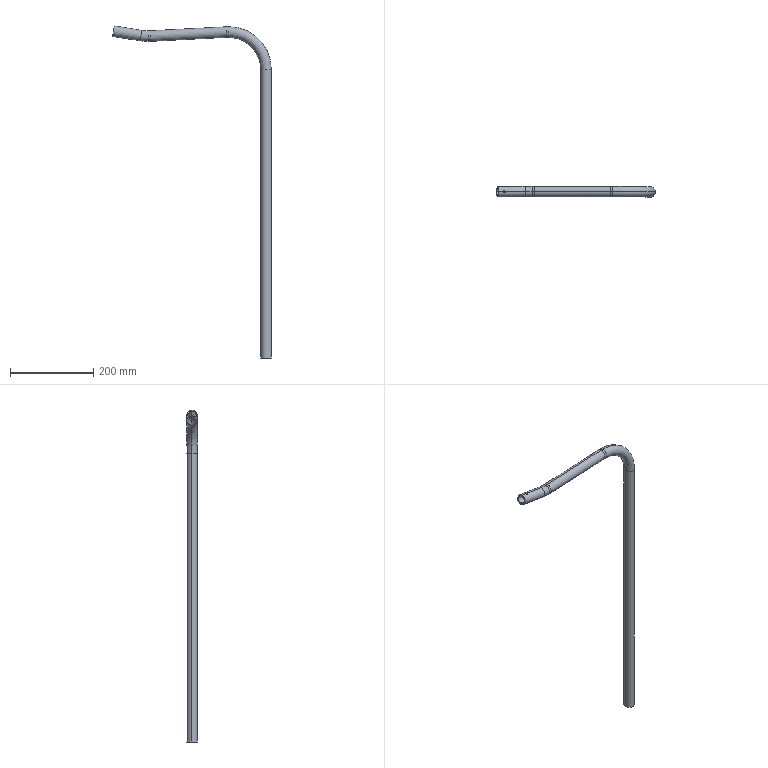Part | STEP file | PN_0029_Default<As Machined> | 1 solid | 38 faces | box 380.934 x 25.4 x 797.47 mm | volume 220981 mm3 | cylinder 16 | torus 16 | cone 4 | plane 2 | commonest cylinder face diameters 19.8 x6 25.4 x6 4.2 x4
STEP:
#1=CARTESIAN_POINT('',(-19.357,0.,-635.525));
#2=VERTEX_POINT('',#1);
#3=CARTESIAN_POINT('',(-18.145,-1.843,-634.518));
#4=VERTEX_POINT('',#3);
#5=CARTESIAN_POINT('',(-18.751,-0.9215,-635.022));
#6=DIRECTION('',(0.5,-0.76,0.4152));
#7=VECTOR('',#6,1.);
#8=LINE('',#5,#7);
#9=EDGE_CURVE('',#2,#4,#8,.T.);
#10=ORIENTED_EDGE('',*,*,#9,.T.);
#11=CARTESIAN_POINT('',(-18.145,1.843,-636.532));
#12=VERTEX_POINT('',#11);
#13=CARTESIAN_POINT('',(-18.145,0.,-635.525));
#14=DIRECTION('',(1.,0.,0.));
#15=AXIS2_PLACEMENT_3D('',#13,#14,$);
#16=CIRCLE('',#15,2.1);
#17=EDGE_CURVE('',#12,#4,#16,.F.);
#18=ORIENTED_EDGE('',*,*,#17,.F.);
#19=CARTESIAN_POINT('',(-18.751,0.9215,-636.028));
#20=DIRECTION('',(0.5,0.76,-0.4152));
#21=VECTOR('',#20,1.);
#22=LINE('',#19,#21);
#23=EDGE_CURVE('',#2,#12,#22,.T.);
#24=ORIENTED_EDGE('',*,*,#23,.F.);
#25=EDGE_LOOP('',(#10,#18,#24));
#26=FACE_OUTER_BOUND('',#25,.T.);
#27=CARTESIAN_POINT('',(-19.357,0.,-635.525));
#28=DIRECTION('',(1.,0.,0.));
#29=DIRECTION('',(0.,0.8776,-0.4794));
#30=AXIS2_PLACEMENT_3D('',#27,#28,#29);
#31=CONICAL_SURFACE('',#30,0.,1.047);
#32=ADVANCED_FACE('',(#26),#31,.F.);
#33=CARTESIAN_POINT('',(-17.145,0.,37.475));
#34=VERTEX_POINT('',#33);
#35=CARTESIAN_POINT('',(-17.145,0.,-633.425));
#36=VERTEX_POINT('',#35);
#37=CARTESIAN_POINT('',(-17.145,0.,37.475));
#38=DIRECTION('',(0.,0.,-1.));
#39=VECTOR('',#38,1.);
#40=LINE('',#37,#39);
#41=EDGE_CURVE('',#34,#36,#40,.T.);
#42=ORIENTED_EDGE('',*,*,#41,.F.);
#43=CARTESIAN_POINT('',(-42.545,0.,37.475));
#44=VERTEX_POINT('',#43);
#45=CARTESIAN_POINT('',(-29.845,0.,37.475));
#46=DIRECTION('',(0.,0.,-1.));
#47=AXIS2_PLACEMENT_3D('',#45,#46,$);
#48=CIRCLE('',#47,12.7);
#49=EDGE_CURVE('',#34,#44,#48,.T.);
#50=ORIENTED_EDGE('',*,*,#49,.T.);
#51=CARTESIAN_POINT('',(-42.545,0.,-655.525));
#52=VERTEX_POINT('',#51);
#53=CARTESIAN_POINT('',(-42.545,0.,37.475));
#54=DIRECTION('',(0.,0.,-1.));
#55=VECTOR('',#54,1.);
#56=LINE('',#53,#55);
#57=EDGE_CURVE('',#44,#52,#56,.T.);
#58=ORIENTED_EDGE('',*,*,#57,.T.);
#59=CARTESIAN_POINT('',(-17.145,0.,-655.525));
#60=VERTEX_POINT('',#59);
#61=CARTESIAN_POINT('',(-29.845,0.,-655.525));
#62=DIRECTION('',(0.,0.,-1.));
#63=AXIS2_PLACEMENT_3D('',#61,#62,$);
#64=CIRCLE('',#63,12.7);
#65=EDGE_CURVE('',#60,#52,#64,.T.);
#66=ORIENTED_EDGE('',*,*,#65,.F.);
#67=CARTESIAN_POINT('',(-17.145,0.,-637.625));
#68=VERTEX_POINT('',#67);
#69=CARTESIAN_POINT('',(-17.145,0.,37.475));
#70=DIRECTION('',(0.,0.,-1.));
#71=VECTOR('',#70,1.);
#72=LINE('',#69,#71);
#73=EDGE_CURVE('',#68,#60,#72,.T.);
#74=ORIENTED_EDGE('',*,*,#73,.F.);
#75=CARTESIAN_POINT('',(-17.279,-1.843,-634.518));
#76=VERTEX_POINT('',#75);
#77=CARTESIAN_POINT('',(-17.279,-1.843,-634.518));
#78=CARTESIAN_POINT('',(-17.34,-2.259,-635.281));
#79=CARTESIAN_POINT('',(-17.369,-2.286,-636.267));
#80=CARTESIAN_POINT('',(-17.221,-1.743,-637.175));
#81=CARTESIAN_POINT('',(-17.145,-0.871,-637.625));
#82=CARTESIAN_POINT('',(-17.145,0.,-637.625));
#83=B_SPLINE_CURVE_WITH_KNOTS('',5,(#77,#78,#79,#80,#81,#82),.UNSPECIFIED.,.F.,.U.,(6,6),(0.,6.159),.UNSPECIFIED.);
#84=EDGE_CURVE('',#76,#68,#83,.T.);
#85=ORIENTED_EDGE('',*,*,#84,.F.);
#86=CARTESIAN_POINT('',(-17.279,-1.843,-634.518));
#87=CARTESIAN_POINT('',(-17.24,-1.574,-634.025));
#88=CARTESIAN_POINT('',(-17.18,-1.128,-633.628));
#89=CARTESIAN_POINT('',(-17.145,-0.5633,-633.425));
#90=CARTESIAN_POINT('',(-17.145,0.,-633.425));
#91=B_SPLINE_CURVE_WITH_KNOTS('',4,(#86,#87,#88,#89,#90),.UNSPECIFIED.,.F.,.U.,(5,5),(0.,3.187),.UNSPECIFIED.);
#92=EDGE_CURVE('',#76,#36,#91,.T.);
#93=ORIENTED_EDGE('',*,*,#92,.T.);
#94=EDGE_LOOP('',(#42,#50,#58,#66,#74,#85,#93));
#95=FACE_OUTER_BOUND('',#94,.T.);
#96=CARTESIAN_POINT('',(-29.845,0.,37.475));
#97=DIRECTION('',(0.,0.,-1.));
#98=DIRECTION('',(1.,0.,0.));
#99=AXIS2_PLACEMENT_3D('',#96,#97,#98);
#100=CYLINDRICAL_SURFACE('',#99,12.7);
#101=ADVANCED_FACE('',(#95),#100,.T.);
#102=CARTESIAN_POINT('',(-119.845,0.,140.175));
#103=VERTEX_POINT('',#102);
#104=CARTESIAN_POINT('',(-119.845,0.,37.475));
#105=DIRECTION('',(0.,1.,0.));
#106=AXIS2_PLACEMENT_3D('',#104,#105,$);
#107=CIRCLE('',#106,102.7);
#108=EDGE_CURVE('',#103,#34,#107,.T.);
#109=ORIENTED_EDGE('',*,*,#108,.F.);
#110=CARTESIAN_POINT('',(-119.845,0.,114.775));
#111=VERTEX_POINT('',#110);
#112=CARTESIAN_POINT('',(-119.845,0.,127.475));
#113=DIRECTION('',(-1.,0.,0.));
#114=AXIS2_PLACEMENT_3D('',#112,#113,$);
#115=CIRCLE('',#114,12.7);
#116=EDGE_CURVE('',#111,#103,#115,.T.);
#117=ORIENTED_EDGE('',*,*,#116,.F.);
#118=CARTESIAN_POINT('',(-119.845,0.,37.475));
#119=DIRECTION('',(0.,1.,0.));
#120=AXIS2_PLACEMENT_3D('',#118,#119,$);
#121=CIRCLE('',#120,77.3);
#122=EDGE_CURVE('',#111,#44,#121,.T.);
#123=ORIENTED_EDGE('',*,*,#122,.T.);
#124=ORIENTED_EDGE('',*,*,#49,.F.);
#125=EDGE_LOOP('',(#109,#117,#123,#124));
#126=FACE_OUTER_BOUND('',#125,.T.);
#127=CARTESIAN_POINT('',(-119.845,0.,37.475));
#128=DIRECTION('',(0.,1.,0.));
#129=DIRECTION('',(0.,0.,1.));
#130=AXIS2_PLACEMENT_3D('',#127,#128,#129);
#131=TOROIDAL_SURFACE('',#130,90.,12.7);
#132=ADVANCED_FACE('',(#126),#131,.T.);
#133=CARTESIAN_POINT('',(-39.745,0.,37.475));
#134=VERTEX_POINT('',#133);
#135=CARTESIAN_POINT('',(-19.945,0.,37.475));
#136=VERTEX_POINT('',#135);
#137=CARTESIAN_POINT('',(-29.845,0.,37.475));
#138=DIRECTION('',(0.,0.,-1.));
#139=AXIS2_PLACEMENT_3D('',#137,#138,$);
#140=CIRCLE('',#139,9.9);
#141=EDGE_CURVE('',#134,#136,#140,.F.);
#142=ORIENTED_EDGE('',*,*,#141,.T.);
#143=CARTESIAN_POINT('',(-19.945,0.,-655.525));
#144=VERTEX_POINT('',#143);
#145=CARTESIAN_POINT('',(-19.945,0.,37.475));
#146=DIRECTION('',(0.,0.,-1.));
#147=VECTOR('',#146,1.);
#148=LINE('',#145,#147);
#149=EDGE_CURVE('',#136,#144,#148,.T.);
#150=ORIENTED_EDGE('',*,*,#149,.T.);
#151=CARTESIAN_POINT('',(-39.745,0.,-655.525));
#152=VERTEX_POINT('',#151);
#153=CARTESIAN_POINT('',(-29.845,0.,-655.525));
#154=DIRECTION('',(0.,0.,-1.));
#155=AXIS2_PLACEMENT_3D('',#153,#154,$);
#156=CIRCLE('',#155,9.9);
#157=EDGE_CURVE('',#152,#144,#156,.F.);
#158=ORIENTED_EDGE('',*,*,#157,.F.);
#159=CARTESIAN_POINT('',(-39.745,0.,37.475));
#160=DIRECTION('',(0.,0.,-1.));
#161=VECTOR('',#160,1.);
#162=LINE('',#159,#161);
#163=EDGE_CURVE('',#134,#152,#162,.T.);
#164=ORIENTED_EDGE('',*,*,#163,.F.);
#165=EDGE_LOOP('',(#142,#150,#158,#164));
#166=FACE_OUTER_BOUND('',#165,.T.);
#167=CARTESIAN_POINT('',(-29.845,0.,37.475));
#168=DIRECTION('',(0.,0.,-1.));
#169=DIRECTION('',(1.,0.,0.));
#170=AXIS2_PLACEMENT_3D('',#167,#168,#169);
#171=CYLINDRICAL_SURFACE('',#170,9.9);
#172=ADVANCED_FACE('',(#166),#171,.F.);
#173=ORIENTED_EDGE('',*,*,#149,.F.);
#174=CARTESIAN_POINT('',(-29.845,0.,37.475));
#175=DIRECTION('',(0.,0.,-1.));
#176=AXIS2_PLACEMENT_3D('',#174,#175,$);
#177=CIRCLE('',#176,9.9);
#178=EDGE_CURVE('',#136,#134,#177,.F.);
#179=ORIENTED_EDGE('',*,*,#178,.T.);
#180=ORIENTED_EDGE('',*,*,#163,.T.);
#181=CARTESIAN_POINT('',(-29.845,0.,-655.525));
#182=DIRECTION('',(0.,0.,-1.));
#183=AXIS2_PLACEMENT_3D('',#181,#182,$);
#184=CIRCLE('',#183,9.9);
#185=EDGE_CURVE('',#144,#152,#184,.F.);
#186=ORIENTED_EDGE('',*,*,#185,.F.);
#187=EDGE_LOOP('',(#173,#179,#180,#186));
#188=FACE_OUTER_BOUND('',#187,.T.);
#189=CARTESIAN_POINT('',(-29.845,0.,37.475));
#190=DIRECTION('',(0.,0.,-1.));
#191=DIRECTION('',(-1.,0.,0.));
#192=AXIS2_PLACEMENT_3D('',#189,#190,#191);
#193=CYLINDRICAL_SURFACE('',#192,9.9);
#194=ADVANCED_FACE('',(#188),#193,.F.);
#195=CARTESIAN_POINT('',(-119.845,0.,117.575));
#196=VERTEX_POINT('',#195);
#197=CARTESIAN_POINT('',(-119.845,0.,137.375));
#198=VERTEX_POINT('',#197);
#199=CARTESIAN_POINT('',(-119.845,0.,127.475));
#200=DIRECTION('',(-1.,0.,0.));
#201=AXIS2_PLACEMENT_3D('',#199,#200,$);
#202=CIRCLE('',#201,9.9);
#203=EDGE_CURVE('',#196,#198,#202,.T.);
#204=ORIENTED_EDGE('',*,*,#203,.T.);
#205=CARTESIAN_POINT('',(-119.845,0.,37.475));
#206=DIRECTION('',(0.,1.,0.));
#207=AXIS2_PLACEMENT_3D('',#205,#206,$);
#208=CIRCLE('',#207,99.9);
#209=EDGE_CURVE('',#198,#136,#208,.T.);
#210=ORIENTED_EDGE('',*,*,#209,.T.);
#211=ORIENTED_EDGE('',*,*,#141,.F.);
#212=CARTESIAN_POINT('',(-119.845,0.,37.475));
#213=DIRECTION('',(0.,1.,0.));
#214=AXIS2_PLACEMENT_3D('',#212,#213,$);
#215=CIRCLE('',#214,80.1);
#216=EDGE_CURVE('',#196,#134,#215,.T.);
#217=ORIENTED_EDGE('',*,*,#216,.F.);
#218=EDGE_LOOP('',(#204,#210,#211,#217));
#219=FACE_OUTER_BOUND('',#218,.T.);
#220=CARTESIAN_POINT('',(-119.845,0.,37.475));
#221=DIRECTION('',(0.,1.,0.));
#222=DIRECTION('',(0.,0.,1.));
#223=AXIS2_PLACEMENT_3D('',#220,#221,#222);
#224=TOROIDAL_SURFACE('',#223,90.,9.9);
#225=ADVANCED_FACE('',(#219),#224,.F.);
#226=ORIENTED_EDGE('',*,*,#209,.F.);
#227=CARTESIAN_POINT('',(-119.845,0.,127.475));
#228=DIRECTION('',(-1.,0.,0.));
#229=AXIS2_PLACEMENT_3D('',#227,#228,$);
#230=CIRCLE('',#229,9.9);
#231=EDGE_CURVE('',#198,#196,#230,.T.);
#232=ORIENTED_EDGE('',*,*,#231,.T.);
#233=ORIENTED_EDGE('',*,*,#216,.T.);
#234=ORIENTED_EDGE('',*,*,#178,.F.);
#235=EDGE_LOOP('',(#226,#232,#233,#234));
#236=FACE_OUTER_BOUND('',#235,.T.);
#237=CARTESIAN_POINT('',(-119.845,0.,37.475));
#238=DIRECTION('',(0.,1.,0.));
#239=DIRECTION('',(0.,0.,1.));
#240=AXIS2_PLACEMENT_3D('',#237,#238,#239);
#241=TOROIDAL_SURFACE('',#240,90.,9.9);
#242=ADVANCED_FACE('',(#236),#241,.F.);
#243=CARTESIAN_POINT('',(-124.037,0.,117.465));
#244=VERTEX_POINT('',#243);
#245=CARTESIAN_POINT('',(-125.073,0.,137.238));
#246=VERTEX_POINT('',#245);
#247=CARTESIAN_POINT('',(-124.555,0.,127.352));
#248=DIRECTION('',(-0.9986,0.,-0.05234));
#249=AXIS2_PLACEMENT_3D('',#247,#248,$);
#250=CIRCLE('',#249,9.9);
#251=EDGE_CURVE('',#244,#246,#250,.T.);
#252=ORIENTED_EDGE('',*,*,#251,.T.);
#253=CARTESIAN_POINT('',(-119.845,0.,37.475));
#254=DIRECTION('',(0.,1.,0.));
#255=AXIS2_PLACEMENT_3D('',#253,#254,$);
#256=CIRCLE('',#255,99.9);
#257=EDGE_CURVE('',#246,#198,#256,.T.);
#258=ORIENTED_EDGE('',*,*,#257,.T.);
#259=ORIENTED_EDGE('',*,*,#203,.F.);
#260=CARTESIAN_POINT('',(-119.845,0.,37.475));
#261=DIRECTION('',(0.,1.,0.));
#262=AXIS2_PLACEMENT_3D('',#260,#261,$);
#263=CIRCLE('',#262,80.1);
#264=EDGE_CURVE('',#244,#196,#263,.T.);
#265=ORIENTED_EDGE('',*,*,#264,.F.);
#266=EDGE_LOOP('',(#252,#258,#259,#265));
#267=FACE_OUTER_BOUND('',#266,.T.);
#268=CARTESIAN_POINT('',(-119.845,0.,37.475));
#269=DIRECTION('',(0.,1.,0.));
#270=DIRECTION('',(0.,0.,-1.));
#271=AXIS2_PLACEMENT_3D('',#268,#269,#270);
#272=TOROIDAL_SURFACE('',#271,90.,9.9);
#273=ADVANCED_FACE('',(#267),#272,.F.);
#274=ORIENTED_EDGE('',*,*,#257,.F.);
#275=CARTESIAN_POINT('',(-124.555,0.,127.352));
#276=DIRECTION('',(-0.9986,0.,-0.05234));
#277=AXIS2_PLACEMENT_3D('',#275,#276,$);
#278=CIRCLE('',#277,9.9);
#279=EDGE_CURVE('',#246,#244,#278,.T.);
#280=ORIENTED_EDGE('',*,*,#279,.T.);
#281=ORIENTED_EDGE('',*,*,#264,.T.);
#282=ORIENTED_EDGE('',*,*,#231,.F.);
#283=EDGE_LOOP('',(#274,#280,#281,#282));
#284=FACE_OUTER_BOUND('',#283,.T.);
#285=CARTESIAN_POINT('',(-119.845,0.,37.475));
#286=DIRECTION('',(0.,1.,0.));
#287=DIRECTION('',(0.,0.,-1.));
#288=AXIS2_PLACEMENT_3D('',#285,#286,#287);
#289=TOROIDAL_SURFACE('',#288,90.,9.9);
#290=ADVANCED_FACE('',(#284),#289,.F.);
#291=CARTESIAN_POINT('',(-306.794,0.,107.887));
#292=VERTEX_POINT('',#291);
#293=CARTESIAN_POINT('',(-307.83,0.,127.66));
#294=VERTEX_POINT('',#293);
#295=CARTESIAN_POINT('',(-307.312,0.,117.774));
#296=DIRECTION('',(0.9986,0.,0.05234));
#297=AXIS2_PLACEMENT_3D('',#295,#296,$);
#298=CIRCLE('',#297,9.9);
#299=EDGE_CURVE('',#292,#294,#298,.F.);
#300=ORIENTED_EDGE('',*,*,#299,.T.);
#301=CARTESIAN_POINT('',(-307.83,0.,127.66));
#302=DIRECTION('',(0.9986,0.,0.05234));
#303=VECTOR('',#302,1.);
#304=LINE('',#301,#303);
#305=EDGE_CURVE('',#294,#246,#304,.T.);
#306=ORIENTED_EDGE('',*,*,#305,.T.);
#307=ORIENTED_EDGE('',*,*,#251,.F.);
#308=CARTESIAN_POINT('',(-306.794,0.,107.887));
#309=DIRECTION('',(0.9986,0.,0.05234));
#310=VECTOR('',#309,1.);
#311=LINE('',#308,#310);
#312=EDGE_CURVE('',#292,#244,#311,.T.);
#313=ORIENTED_EDGE('',*,*,#312,.F.);
#314=EDGE_LOOP('',(#300,#306,#307,#313));
#315=FACE_OUTER_BOUND('',#314,.T.);
#316=CARTESIAN_POINT('',(-307.312,0.,117.774));
#317=DIRECTION('',(0.9986,0.,0.05234));
#318=DIRECTION('',(-0.05234,0.,0.9986));
#319=AXIS2_PLACEMENT_3D('',#316,#317,#318);
#320=CYLINDRICAL_SURFACE('',#319,9.9);
#321=ADVANCED_FACE('',(#315),#320,.F.);
#322=ORIENTED_EDGE('',*,*,#305,.F.);
#323=CARTESIAN_POINT('',(-307.312,0.,117.774));
#324=DIRECTION('',(0.9986,0.,0.05234));
#325=AXIS2_PLACEMENT_3D('',#323,#324,$);
#326=CIRCLE('',#325,9.9);
#327=EDGE_CURVE('',#294,#292,#326,.F.);
#328=ORIENTED_EDGE('',*,*,#327,.T.);
#329=ORIENTED_EDGE('',*,*,#312,.T.);
#330=ORIENTED_EDGE('',*,*,#279,.F.);
#331=EDGE_LOOP('',(#322,#328,#329,#330));
#332=FACE_OUTER_BOUND('',#331,.T.);
#333=CARTESIAN_POINT('',(-307.312,0.,117.774));
#334=DIRECTION('',(0.9986,0.,0.05234));
#335=DIRECTION('',(0.05234,0.,-0.9986));
#336=AXIS2_PLACEMENT_3D('',#333,#334,#335);
#337=CYLINDRICAL_SURFACE('',#336,9.9);
#338=ADVANCED_FACE('',(#332),#337,.F.);
#339=CARTESIAN_POINT('',(-313.069,0.,107.723));
#340=VERTEX_POINT('',#339);
#341=CARTESIAN_POINT('',(-313.069,0.,227.623));
#342=DIRECTION('',(0.,-1.,0.));
#343=AXIS2_PLACEMENT_3D('',#341,#342,$);
#344=CIRCLE('',#343,119.9);
#345=EDGE_CURVE('',#340,#292,#344,.T.);
#346=ORIENTED_EDGE('',*,*,#345,.F.);
#347=CARTESIAN_POINT('',(-313.069,0.,127.523));
#348=VERTEX_POINT('',#347);
#349=CARTESIAN_POINT('',(-313.069,0.,117.623));
#350=DIRECTION('',(-1.,0.,0.));
#351=AXIS2_PLACEMENT_3D('',#349,#350,$);
#352=CIRCLE('',#351,9.9);
#353=EDGE_CURVE('',#340,#348,#352,.T.);
#354=ORIENTED_EDGE('',*,*,#353,.T.);
#355=CARTESIAN_POINT('',(-313.069,0.,227.623));
#356=DIRECTION('',(0.,-1.,0.));
#357=AXIS2_PLACEMENT_3D('',#355,#356,$);
#358=CIRCLE('',#357,100.1);
#359=EDGE_CURVE('',#348,#294,#358,.T.);
#360=ORIENTED_EDGE('',*,*,#359,.T.);
#361=ORIENTED_EDGE('',*,*,#299,.F.);
#362=EDGE_LOOP('',(#346,#354,#360,#361));
#363=FACE_OUTER_BOUND('',#362,.T.);
#364=CARTESIAN_POINT('',(-313.069,0.,227.623));
#365=DIRECTION('',(0.,-1.,0.));
#366=DIRECTION('',(0.,0.,-1.));
#367=AXIS2_PLACEMENT_3D('',#364,#365,#366);
#368=TOROIDAL_SURFACE('',#367,110.,9.9);
#369=ADVANCED_FACE('',(#363),#368,.F.);
#370=CARTESIAN_POINT('',(-313.069,0.,117.623));
#371=DIRECTION('',(-1.,0.,0.));
#372=AXIS2_PLACEMENT_3D('',#370,#371,$);
#373=CIRCLE('',#372,9.9);
#374=EDGE_CURVE('',#348,#340,#373,.T.);
#375=ORIENTED_EDGE('',*,*,#374,.T.);
#376=ORIENTED_EDGE('',*,*,#345,.T.);
#377=ORIENTED_EDGE('',*,*,#327,.F.);
#378=ORIENTED_EDGE('',*,*,#359,.F.);
#379=EDGE_LOOP('',(#375,#376,#377,#378));
#380=FACE_OUTER_BOUND('',#379,.T.);
#381=CARTESIAN_POINT('',(-313.069,0.,227.623));
#382=DIRECTION('',(0.,-1.,0.));
#383=DIRECTION('',(0.,0.,-1.));
#384=AXIS2_PLACEMENT_3D('',#381,#382,#383);
#385=TOROIDAL_SURFACE('',#384,110.,9.9);
#386=ADVANCED_FACE('',(#380),#385,.F.);
#387=CARTESIAN_POINT('',(-331.825,0.,109.199));
#388=VERTEX_POINT('',#387);
#389=CARTESIAN_POINT('',(-313.069,0.,227.623));
#390=DIRECTION('',(0.,-1.,0.));
#391=AXIS2_PLACEMENT_3D('',#389,#390,$);
#392=CIRCLE('',#391,119.9);
#393=EDGE_CURVE('',#388,#340,#392,.T.);
#394=ORIENTED_EDGE('',*,*,#393,.F.);
#395=CARTESIAN_POINT('',(-328.728,0.,128.755));
#396=VERTEX_POINT('',#395);
#397=CARTESIAN_POINT('',(-330.276,0.,118.977));
#398=DIRECTION('',(-0.9877,0.,0.1564));
#399=AXIS2_PLACEMENT_3D('',#397,#398,$);
#400=CIRCLE('',#399,9.9);
#401=EDGE_CURVE('',#388,#396,#400,.T.);
#402=ORIENTED_EDGE('',*,*,#401,.T.);
#403=CARTESIAN_POINT('',(-313.069,0.,227.623));
#404=DIRECTION('',(0.,-1.,0.));
#405=AXIS2_PLACEMENT_3D('',#403,#404,$);
#406=CIRCLE('',#405,100.1);
#407=EDGE_CURVE('',#396,#348,#406,.T.);
#408=ORIENTED_EDGE('',*,*,#407,.T.);
#409=ORIENTED_EDGE('',*,*,#353,.F.);
#410=EDGE_LOOP('',(#394,#402,#408,#409));
#411=FACE_OUTER_BOUND('',#410,.T.);
#412=CARTESIAN_POINT('',(-313.069,0.,227.623));
#413=DIRECTION('',(0.,-1.,0.));
#414=DIRECTION('',(0.,0.,1.));
#415=AXIS2_PLACEMENT_3D('',#412,#413,#414);
#416=TOROIDAL_SURFACE('',#415,110.,9.9);
#417=ADVANCED_FACE('',(#411),#416,.F.);
#418=CARTESIAN_POINT('',(-330.276,0.,118.977));
#419=DIRECTION('',(-0.9877,0.,0.1564));
#420=AXIS2_PLACEMENT_3D('',#418,#419,$);
#421=CIRCLE('',#420,9.9);
#422=EDGE_CURVE('',#396,#388,#421,.T.);
#423=ORIENTED_EDGE('',*,*,#422,.T.);
#424=ORIENTED_EDGE('',*,*,#393,.T.);
#425=ORIENTED_EDGE('',*,*,#374,.F.);
#426=ORIENTED_EDGE('',*,*,#407,.F.);
#427=EDGE_LOOP('',(#423,#424,#425,#426));
#428=FACE_OUTER_BOUND('',#427,.T.);
#429=CARTESIAN_POINT('',(-313.069,0.,227.623));
#430=DIRECTION('',(0.,-1.,0.));
#431=DIRECTION('',(0.,0.,1.));
#432=AXIS2_PLACEMENT_3D('',#429,#430,#431);
#433=TOROIDAL_SURFACE('',#432,110.,9.9);
#434=ADVANCED_FACE('',(#428),#433,.F.);
#435=CARTESIAN_POINT('',(-394.544,0.,139.18));
#436=VERTEX_POINT('',#435);
#437=CARTESIAN_POINT('',(-397.641,0.,119.623));
#438=VERTEX_POINT('',#437);
#439=CARTESIAN_POINT('',(-394.544,0.,139.18));
#440=CARTESIAN_POINT('',(-394.544,-1.555,139.18));
#441=CARTESIAN_POINT('',(-394.591,-3.11,138.878));
#442=CARTESIAN_POINT('',(-394.687,-4.585,138.275));
#443=CARTESIAN_POINT('',(-394.964,-7.216,136.529));
#444=CARTESIAN_POINT('',(-395.375,-8.984,133.93));
#445=CARTESIAN_POINT('',(-395.606,-9.595,132.473));
#446=CARTESIAN_POINT('',(-396.092,-10.205,129.402));
#447=CARTESIAN_POINT('',(-396.579,-9.595,126.33));
#448=CARTESIAN_POINT('',(-396.81,-8.984,124.873));
#449=CARTESIAN_POINT('',(-397.221,-7.216,122.274));
#450=CARTESIAN_POINT('',(-397.498,-4.585,120.528));
#451=CARTESIAN_POINT('',(-397.593,-3.11,119.925));
#452=CARTESIAN_POINT('',(-397.641,-1.555,119.623));
#453=CARTESIAN_POINT('',(-397.641,0.,119.623));
#454=B_SPLINE_CURVE_WITH_KNOTS('',5,(#439,#440,#441,#442,#443,#444,#445,#446,#447,#448,#449,#450,#451,#452,#453),.UNSPECIFIED.,.F.,.U.,(6,3,3,3,6),(-15.551,-7.775,0.,7.775,15.551),.UNSPECIFIED.);
#455=EDGE_CURVE('',#436,#438,#454,.T.);
#456=ORIENTED_EDGE('',*,*,#455,.F.);
#457=CARTESIAN_POINT('',(-368.235,0.,135.013));
#458=DIRECTION('',(0.9877,0.,-0.1564));
#459=VECTOR('',#458,1.);
#460=LINE('',#457,#459);
#461=EDGE_CURVE('',#436,#396,#460,.T.);
#462=ORIENTED_EDGE('',*,*,#461,.T.);
#463=ORIENTED_EDGE('',*,*,#401,.F.);
#464=CARTESIAN_POINT('',(-371.333,0.,115.457));
#465=DIRECTION('',(0.9877,0.,-0.1564));
#466=VECTOR('',#465,1.);
#467=LINE('',#464,#466);
#468=EDGE_CURVE('',#438,#388,#467,.T.);
#469=ORIENTED_EDGE('',*,*,#468,.F.);
#470=EDGE_LOOP('',(#456,#462,#463,#469));
#471=FACE_OUTER_BOUND('',#470,.T.);
#472=CARTESIAN_POINT('',(-369.784,0.,125.235));
#473=DIRECTION('',(0.9877,0.,-0.1564));
#474=DIRECTION('',(0.1564,0.,0.9877));
#475=AXIS2_PLACEMENT_3D('',#472,#473,#474);
#476=CYLINDRICAL_SURFACE('',#475,9.9);
#477=ADVANCED_FACE('',(#471),#476,.F.);
#478=ORIENTED_EDGE('',*,*,#461,.F.);
#479=CARTESIAN_POINT('',(-397.641,0.,119.623));
#480=CARTESIAN_POINT('',(-397.641,1.555,119.623));
#481=CARTESIAN_POINT('',(-397.593,3.11,119.925));
#482=CARTESIAN_POINT('',(-397.498,4.585,120.528));
#483=CARTESIAN_POINT('',(-397.221,7.216,122.274));
#484=CARTESIAN_POINT('',(-396.81,8.984,124.873));
#485=CARTESIAN_POINT('',(-396.579,9.595,126.33));
#486=CARTESIAN_POINT('',(-396.092,10.205,129.402));
#487=CARTESIAN_POINT('',(-395.606,9.595,132.473));
#488=CARTESIAN_POINT('',(-395.375,8.984,133.93));
#489=CARTESIAN_POINT('',(-394.964,7.216,136.529));
#490=CARTESIAN_POINT('',(-394.687,4.585,138.275));
#491=CARTESIAN_POINT('',(-394.591,3.11,138.878));
#492=CARTESIAN_POINT('',(-394.544,1.555,139.18));
#493=CARTESIAN_POINT('',(-394.544,0.,139.18));
#494=B_SPLINE_CURVE_WITH_KNOTS('',5,(#479,#480,#481,#482,#483,#484,#485,#486,#487,#488,#489,#490,#491,#492,#493),.UNSPECIFIED.,.F.,.U.,(6,3,3,3,6),(-15.551,-7.775,0.,7.775,15.551),.UNSPECIFIED.);
#495=EDGE_CURVE('',#438,#436,#494,.T.);
#496=ORIENTED_EDGE('',*,*,#495,.F.);
#497=ORIENTED_EDGE('',*,*,#468,.T.);
#498=ORIENTED_EDGE('',*,*,#422,.F.);
#499=EDGE_LOOP('',(#478,#496,#497,#498));
#500=FACE_OUTER_BOUND('',#499,.T.);
#501=CARTESIAN_POINT('',(-369.784,0.,125.235));
#502=DIRECTION('',(0.9877,0.,-0.1564));
#503=DIRECTION('',(-0.1564,0.,-0.9877));
#504=AXIS2_PLACEMENT_3D('',#501,#502,#503);
#505=CYLINDRICAL_SURFACE('',#504,9.9);
#506=ADVANCED_FACE('',(#500),#505,.F.);
#507=CARTESIAN_POINT('',(-307.976,0.,130.456));
#508=VERTEX_POINT('',#507);
#509=CARTESIAN_POINT('',(-125.22,0.,140.034));
#510=VERTEX_POINT('',#509);
#511=CARTESIAN_POINT('',(-307.976,0.,130.456));
#512=DIRECTION('',(0.9986,0.,0.05234));
#513=VECTOR('',#512,1.);
#514=LINE('',#511,#513);
#515=EDGE_CURVE('',#508,#510,#514,.T.);
#516=ORIENTED_EDGE('',*,*,#515,.F.);
#517=CARTESIAN_POINT('',(-306.647,0.,105.091));
#518=VERTEX_POINT('',#517);
#519=CARTESIAN_POINT('',(-307.312,0.,117.774));
#520=DIRECTION('',(0.9986,0.,0.05234));
#521=AXIS2_PLACEMENT_3D('',#519,#520,$);
#522=CIRCLE('',#521,12.7);
#523=EDGE_CURVE('',#508,#518,#522,.T.);
#524=ORIENTED_EDGE('',*,*,#523,.T.);
#525=CARTESIAN_POINT('',(-123.89,0.,114.669));
#526=VERTEX_POINT('',#525);
#527=CARTESIAN_POINT('',(-306.647,0.,105.091));
#528=DIRECTION('',(0.9986,0.,0.05234));
#529=VECTOR('',#528,1.);
#530=LINE('',#527,#529);
#531=EDGE_CURVE('',#518,#526,#530,.T.);
#532=ORIENTED_EDGE('',*,*,#531,.T.);
#533=CARTESIAN_POINT('',(-125.22,0.,140.034));
#534=CARTESIAN_POINT('',(-125.22,-1.995,140.034));
#535=CARTESIAN_POINT('',(-125.199,-3.99,139.643));
#536=CARTESIAN_POINT('',(-125.158,-5.882,138.86));
#537=CARTESIAN_POINT('',(-125.039,-9.257,136.596));
#538=CARTESIAN_POINT('',(-124.863,-11.525,133.226));
#539=CARTESIAN_POINT('',(-124.764,-12.308,131.336));
#540=CARTESIAN_POINT('',(-124.555,-13.092,127.352));
#541=CARTESIAN_POINT('',(-124.346,-12.308,123.367));
#542=CARTESIAN_POINT('',(-124.247,-11.525,121.478));
#543=CARTESIAN_POINT('',(-124.07,-9.257,118.107));
#544=CARTESIAN_POINT('',(-123.952,-5.882,115.843));
#545=CARTESIAN_POINT('',(-123.911,-3.99,115.06));
#546=CARTESIAN_POINT('',(-123.89,-1.995,114.669));
#547=CARTESIAN_POINT('',(-123.89,0.,114.669));
#548=B_SPLINE_CURVE_WITH_KNOTS('',5,(#533,#534,#535,#536,#537,#538,#539,#540,#541,#542,#543,#544,#545,#546,#547),.UNSPECIFIED.,.F.,.U.,(6,3,3,3,6),(-19.949,-9.975,0.,9.975,19.949),.UNSPECIFIED.);
#549=EDGE_CURVE('',#510,#526,#548,.T.);
#550=ORIENTED_EDGE('',*,*,#549,.F.);
#551=EDGE_LOOP('',(#516,#524,#532,#550));
#552=FACE_OUTER_BOUND('',#551,.T.);
#553=CARTESIAN_POINT('',(-307.312,0.,117.774));
#554=DIRECTION('',(0.9986,0.,0.05234));
#555=DIRECTION('',(-0.05234,0.,0.9986));
#556=AXIS2_PLACEMENT_3D('',#553,#554,#555);
#557=CYLINDRICAL_SURFACE('',#556,12.7);
#558=ADVANCED_FACE('',(#552),#557,.T.);
#559=CARTESIAN_POINT('',(-313.069,0.,104.923));
#560=VERTEX_POINT('',#559);
#561=CARTESIAN_POINT('',(-313.069,0.,130.323));
#562=VERTEX_POINT('',#561);
#563=CARTESIAN_POINT('',(-313.069,0.,117.623));
#564=DIRECTION('',(-1.,0.,0.));
#565=AXIS2_PLACEMENT_3D('',#563,#564,$);
#566=CIRCLE('',#565,12.7);
#567=EDGE_CURVE('',#560,#562,#566,.T.);
#568=ORIENTED_EDGE('',*,*,#567,.F.);
#569=CARTESIAN_POINT('',(-313.069,0.,227.623));
#570=DIRECTION('',(0.,-1.,0.));
#571=AXIS2_PLACEMENT_3D('',#569,#570,$);
#572=CIRCLE('',#571,122.7);
#573=EDGE_CURVE('',#560,#518,#572,.T.);
#574=ORIENTED_EDGE('',*,*,#573,.T.);
#575=ORIENTED_EDGE('',*,*,#523,.F.);
#576=CARTESIAN_POINT('',(-313.069,0.,227.623));
#577=DIRECTION('',(0.,-1.,0.));
#578=AXIS2_PLACEMENT_3D('',#576,#577,$);
#579=CIRCLE('',#578,97.3);
#580=EDGE_CURVE('',#562,#508,#579,.T.);
#581=ORIENTED_EDGE('',*,*,#580,.F.);
#582=EDGE_LOOP('',(#568,#574,#575,#581));
#583=FACE_OUTER_BOUND('',#582,.T.);
#584=CARTESIAN_POINT('',(-313.069,0.,227.623));
#585=DIRECTION('',(0.,-1.,0.));
#586=DIRECTION('',(0.,0.,-1.));
#587=AXIS2_PLACEMENT_3D('',#584,#585,#586);
#588=TOROIDAL_SURFACE('',#587,110.,12.7);
#589=ADVANCED_FACE('',(#583),#588,.T.);
#590=ORIENTED_EDGE('',*,*,#573,.F.);
#591=CARTESIAN_POINT('',(-313.069,0.,117.623));
#592=DIRECTION('',(-1.,0.,0.));
#593=AXIS2_PLACEMENT_3D('',#591,#592,$);
#594=CIRCLE('',#593,12.7);
#595=EDGE_CURVE('',#562,#560,#594,.T.);
#596=ORIENTED_EDGE('',*,*,#595,.F.);
#597=ORIENTED_EDGE('',*,*,#580,.T.);
#598=CARTESIAN_POINT('',(-307.312,0.,117.774));
#599=DIRECTION('',(-0.9986,0.,-0.05234));
#600=AXIS2_PLACEMENT_3D('',#598,#599,$);
#601=CIRCLE('',#600,12.7);
#602=EDGE_CURVE('',#518,#508,#601,.F.);
#603=ORIENTED_EDGE('',*,*,#602,.F.);
#604=EDGE_LOOP('',(#590,#596,#597,#603));
#605=FACE_OUTER_BOUND('',#604,.T.);
#606=CARTESIAN_POINT('',(-313.069,0.,227.623));
#607=DIRECTION('',(0.,-1.,0.));
#608=DIRECTION('',(0.,0.,-1.));
#609=AXIS2_PLACEMENT_3D('',#606,#607,#608);
#610=TOROIDAL_SURFACE('',#609,110.,12.7);
#611=ADVANCED_FACE('',(#605),#610,.T.);
#612=CARTESIAN_POINT('',(-394.106,0.,141.945));
#613=VERTEX_POINT('',#612);
#614=CARTESIAN_POINT('',(-381.364,0.,139.927));
#615=VERTEX_POINT('',#614);
#616=CARTESIAN_POINT('',(-367.797,0.,137.778));
#617=DIRECTION('',(0.9877,0.,-0.1564));
#618=VECTOR('',#617,1.);
#619=LINE('',#616,#618);
#620=EDGE_CURVE('',#613,#615,#619,.T.);
#621=ORIENTED_EDGE('',*,*,#620,.F.);
#622=CARTESIAN_POINT('',(-398.079,0.,116.858));
#623=VERTEX_POINT('',#622);
#624=CARTESIAN_POINT('',(-398.079,0.,116.858));
#625=CARTESIAN_POINT('',(-398.079,-1.995,116.858));
#626=CARTESIAN_POINT('',(-398.018,-3.99,117.245));
#627=CARTESIAN_POINT('',(-397.895,-5.882,118.019));
#628=CARTESIAN_POINT('',(-397.541,-9.257,120.258));
#629=CARTESIAN_POINT('',(-397.013,-11.525,123.592));
#630=CARTESIAN_POINT('',(-396.717,-12.308,125.461));
#631=CARTESIAN_POINT('',(-396.092,-13.092,129.402));
#632=CARTESIAN_POINT('',(-395.468,-12.308,133.342));
#633=CARTESIAN_POINT('',(-395.172,-11.525,135.211));
#634=CARTESIAN_POINT('',(-394.644,-9.257,138.545));
#635=CARTESIAN_POINT('',(-394.29,-5.882,140.784));
#636=CARTESIAN_POINT('',(-394.167,-3.99,141.558));
#637=CARTESIAN_POINT('',(-394.106,-1.995,141.945));
#638=CARTESIAN_POINT('',(-394.106,0.,141.945));
#639=B_SPLINE_CURVE_WITH_KNOTS('',5,(#624,#625,#626,#627,#628,#629,#630,#631,#632,#633,#634,#635,#636,#637,#638),.UNSPECIFIED.,.F.,.U.,(6,3,3,3,6),(-19.949,-9.975,0.,9.975,19.949),.UNSPECIFIED.);
#640=EDGE_CURVE('',#623,#613,#639,.T.);
#641=ORIENTED_EDGE('',*,*,#640,.F.);
#642=CARTESIAN_POINT('',(-332.263,0.,106.434));
#643=VERTEX_POINT('',#642);
#644=CARTESIAN_POINT('',(-371.771,0.,112.691));
#645=DIRECTION('',(0.9877,0.,-0.1564));
#646=VECTOR('',#645,1.);
#647=LINE('',#644,#646);
#648=EDGE_CURVE('',#623,#643,#647,.T.);
#649=ORIENTED_EDGE('',*,*,#648,.T.);
#650=CARTESIAN_POINT('',(-328.29,0.,131.521));
#651=VERTEX_POINT('',#650);
#652=CARTESIAN_POINT('',(-330.276,0.,118.977));
#653=DIRECTION('',(0.9877,0.,-0.1564));
#654=AXIS2_PLACEMENT_3D('',#652,#653,$);
#655=CIRCLE('',#654,12.7);
#656=EDGE_CURVE('',#651,#643,#655,.T.);
#657=ORIENTED_EDGE('',*,*,#656,.F.);
#658=CARTESIAN_POINT('',(-377.216,0.,139.27));
#659=VERTEX_POINT('',#658);
#660=CARTESIAN_POINT('',(-367.797,0.,137.778));
#661=DIRECTION('',(0.9877,0.,-0.1564));
#662=VECTOR('',#661,1.);
#663=LINE('',#660,#662);
#664=EDGE_CURVE('',#659,#651,#663,.T.);
#665=ORIENTED_EDGE('',*,*,#664,.F.);
#666=CARTESIAN_POINT('',(-377.476,-1.007,139.271));
#667=VERTEX_POINT('',#666);
#668=CARTESIAN_POINT('',(-377.476,-1.007,139.271));
#669=CARTESIAN_POINT('',(-377.307,-0.7001,139.269));
#670=CARTESIAN_POINT('',(-377.216,-0.3503,139.27));
#671=CARTESIAN_POINT('',(-377.216,0.,139.27));
#672=B_SPLINE_CURVE_WITH_KNOTS('',3,(#668,#669,#670,#671),.UNSPECIFIED.,.F.,.U.,(4,4),(0.,1.486),.UNSPECIFIED.);
#673=EDGE_CURVE('',#667,#659,#672,.T.);
#674=ORIENTED_EDGE('',*,*,#673,.F.);
#675=CARTESIAN_POINT('',(-377.476,-1.007,139.271));
#676=CARTESIAN_POINT('',(-377.737,-1.478,139.274));
#677=CARTESIAN_POINT('',(-378.148,-1.866,139.286));
#678=CARTESIAN_POINT('',(-378.673,-2.109,139.321));
#679=CARTESIAN_POINT('',(-379.823,-2.226,139.487));
#680=CARTESIAN_POINT('',(-380.802,-1.626,139.738));
#681=CARTESIAN_POINT('',(-381.177,-1.146,139.865));
#682=CARTESIAN_POINT('',(-381.364,-0.5729,139.927));
#683=CARTESIAN_POINT('',(-381.364,0.,139.927));
#684=B_SPLINE_CURVE_WITH_KNOTS('',5,(#675,#676,#677,#678,#679,#680,#681,#682,#683),.UNSPECIFIED.,.F.,.U.,(6,3,6),(0.,3.808,7.86),.UNSPECIFIED.);
#685=EDGE_CURVE('',#667,#615,#684,.T.);
#686=ORIENTED_EDGE('',*,*,#685,.T.);
#687=EDGE_LOOP('',(#621,#641,#649,#657,#665,#674,#686));
#688=FACE_OUTER_BOUND('',#687,.T.);
#689=CARTESIAN_POINT('',(-369.784,0.,125.235));
#690=DIRECTION('',(0.9877,0.,-0.1564));
#691=DIRECTION('',(0.1564,0.,0.9877));
#692=AXIS2_PLACEMENT_3D('',#689,#690,#691);
#693=CYLINDRICAL_SURFACE('',#692,12.7);
#694=ADVANCED_FACE('',(#688),#693,.T.);
#695=ORIENTED_EDGE('',*,*,#664,.T.);
#696=CARTESIAN_POINT('',(-330.276,0.,118.977));
#697=DIRECTION('',(0.9877,0.,-0.1564));
#698=AXIS2_PLACEMENT_3D('',#696,#697,$);
#699=CIRCLE('',#698,12.7);
#700=EDGE_CURVE('',#643,#651,#699,.T.);
#701=ORIENTED_EDGE('',*,*,#700,.F.);
#702=ORIENTED_EDGE('',*,*,#648,.F.);
#703=CARTESIAN_POINT('',(-396.092,0.,129.402));
#704=DIRECTION('',(0.9877,0.,-0.1564));
#705=AXIS2_PLACEMENT_3D('',#703,#704,$);
#706=CIRCLE('',#705,12.7);
#707=EDGE_CURVE('',#613,#623,#706,.F.);
#708=ORIENTED_EDGE('',*,*,#707,.F.);
#709=ORIENTED_EDGE('',*,*,#620,.T.);
#710=CARTESIAN_POINT('',(-381.117,1.007,139.848));
#711=VERTEX_POINT('',#710);
#712=CARTESIAN_POINT('',(-381.117,1.007,139.848));
#713=CARTESIAN_POINT('',(-381.279,0.7001,139.898));
#714=CARTESIAN_POINT('',(-381.364,0.3503,139.927));
#715=CARTESIAN_POINT('',(-381.364,0.,139.927));
#716=B_SPLINE_CURVE_WITH_KNOTS('',3,(#712,#713,#714,#715),.UNSPECIFIED.,.F.,.U.,(4,4),(0.,1.486),.UNSPECIFIED.);
#717=EDGE_CURVE('',#711,#615,#716,.T.);
#718=ORIENTED_EDGE('',*,*,#717,.F.);
#719=CARTESIAN_POINT('',(-381.117,1.007,139.848));
#720=CARTESIAN_POINT('',(-380.868,1.478,139.77));
#721=CARTESIAN_POINT('',(-380.474,1.866,139.654));
#722=CARTESIAN_POINT('',(-379.964,2.109,139.526));
#723=CARTESIAN_POINT('',(-378.818,2.226,139.327));
#724=CARTESIAN_POINT('',(-377.809,1.626,139.264));
#725=CARTESIAN_POINT('',(-377.414,1.146,139.269));
#726=CARTESIAN_POINT('',(-377.216,0.5729,139.27));
#727=CARTESIAN_POINT('',(-377.216,0.,139.27));
#728=B_SPLINE_CURVE_WITH_KNOTS('',5,(#719,#720,#721,#722,#723,#724,#725,#726,#727),.UNSPECIFIED.,.F.,.U.,(6,3,6),(0.,3.808,7.86),.UNSPECIFIED.);
#729=EDGE_CURVE('',#711,#659,#728,.T.);
#730=ORIENTED_EDGE('',*,*,#729,.T.);
#731=EDGE_LOOP('',(#695,#701,#702,#708,#709,#718,#730));
#732=FACE_OUTER_BOUND('',#731,.T.);
#733=CARTESIAN_POINT('',(-369.784,0.,125.235));
#734=DIRECTION('',(0.9877,0.,-0.1564));
#735=DIRECTION('',(-0.1564,0.,-0.9877));
#736=AXIS2_PLACEMENT_3D('',#733,#734,#735);
#737=CYLINDRICAL_SURFACE('',#736,12.7);
#738=ADVANCED_FACE('',(#732),#737,.T.);
#739=ORIENTED_EDGE('',*,*,#717,.T.);
#740=ORIENTED_EDGE('',*,*,#685,.F.);
#741=CARTESIAN_POINT('',(-377.627,-1.007,138.323));
#742=VERTEX_POINT('',#741);
#743=CARTESIAN_POINT('',(-372.509,-1.007,170.632));
#744=DIRECTION('',(-0.1564,0.,-0.9877));
#745=VECTOR('',#744,1.);
#746=LINE('',#743,#745);
#747=EDGE_CURVE('',#742,#667,#746,.F.);
#748=ORIENTED_EDGE('',*,*,#747,.F.);
#749=CARTESIAN_POINT('',(-381.267,1.007,138.899));
#750=VERTEX_POINT('',#749);
#751=CARTESIAN_POINT('',(-379.447,0.,138.611));
#752=DIRECTION('',(-0.1564,0.,-0.9877));
#753=AXIS2_PLACEMENT_3D('',#751,#752,$);
#754=CIRCLE('',#753,2.1);
#755=EDGE_CURVE('',#742,#750,#754,.T.);
#756=ORIENTED_EDGE('',*,*,#755,.T.);
#757=CARTESIAN_POINT('',(-376.15,1.007,171.209));
#758=DIRECTION('',(-0.1564,0.,-0.9877));
#759=VECTOR('',#758,1.);
#760=LINE('',#757,#759);
#761=EDGE_CURVE('',#750,#711,#760,.F.);
#762=ORIENTED_EDGE('',*,*,#761,.T.);
#763=EDGE_LOOP('',(#739,#740,#748,#756,#762));
#764=FACE_OUTER_BOUND('',#763,.T.);
#765=CARTESIAN_POINT('',(-379.306,0.,139.5));
#766=DIRECTION('',(-0.1564,0.,-0.9877));
#767=DIRECTION('',(0.8668,-0.4794,-0.1373));
#768=AXIS2_PLACEMENT_3D('',#765,#766,#767);
#769=CYLINDRICAL_SURFACE('',#768,2.1);
#770=ADVANCED_FACE('',(#764),#769,.F.);
#771=CARTESIAN_POINT('',(-379.636,0.,137.413));
#772=VERTEX_POINT('',#771);
#773=CARTESIAN_POINT('',(-380.452,0.5034,138.156));
#774=DIRECTION('',(-0.6724,0.4152,0.6127));
#775=VECTOR('',#774,1.);
#776=LINE('',#773,#775);
#777=EDGE_CURVE('',#772,#750,#776,.T.);
#778=ORIENTED_EDGE('',*,*,#777,.T.);
#779=ORIENTED_EDGE('',*,*,#755,.F.);
#780=CARTESIAN_POINT('',(-378.631,-0.5034,137.868));
#781=DIRECTION('',(0.8289,-0.4152,0.375));
#782=VECTOR('',#781,1.);
#783=LINE('',#780,#782);
#784=EDGE_CURVE('',#772,#742,#783,.T.);
#785=ORIENTED_EDGE('',*,*,#784,.F.);
#786=EDGE_LOOP('',(#778,#779,#785));
#787=FACE_OUTER_BOUND('',#786,.T.);
#788=CARTESIAN_POINT('',(-379.636,0.,137.413));
#789=DIRECTION('',(0.1564,0.,0.9877));
#790=DIRECTION('',(0.8668,-0.4794,-0.1373));
#791=AXIS2_PLACEMENT_3D('',#788,#789,#790);
#792=CONICAL_SURFACE('',#791,0.,1.047);
#793=ADVANCED_FACE('',(#787),#792,.F.);
#794=ORIENTED_EDGE('',*,*,#784,.T.);
#795=CARTESIAN_POINT('',(-379.447,0.,138.611));
#796=DIRECTION('',(0.1564,0.,0.9877));
#797=AXIS2_PLACEMENT_3D('',#795,#796,$);
#798=CIRCLE('',#797,2.1);
#799=EDGE_CURVE('',#750,#742,#798,.F.);
#800=ORIENTED_EDGE('',*,*,#799,.F.);
#801=ORIENTED_EDGE('',*,*,#777,.F.);
#802=EDGE_LOOP('',(#794,#800,#801));
#803=FACE_OUTER_BOUND('',#802,.T.);
#804=ADVANCED_FACE('',(#803),#792,.F.);
#805=ORIENTED_EDGE('',*,*,#673,.T.);
#806=ORIENTED_EDGE('',*,*,#729,.F.);
#807=ORIENTED_EDGE('',*,*,#761,.F.);
#808=ORIENTED_EDGE('',*,*,#799,.T.);
#809=ORIENTED_EDGE('',*,*,#747,.T.);
#810=EDGE_LOOP('',(#805,#806,#807,#808,#809));
#811=FACE_OUTER_BOUND('',#810,.T.);
#812=ADVANCED_FACE('',(#811),#769,.F.);
#813=CARTESIAN_POINT('',(-313.069,0.,227.623));
#814=DIRECTION('',(0.,-1.,0.));
#815=AXIS2_PLACEMENT_3D('',#813,#814,$);
#816=CIRCLE('',#815,122.7);
#817=EDGE_CURVE('',#643,#560,#816,.T.);
#818=ORIENTED_EDGE('',*,*,#817,.F.);
#819=ORIENTED_EDGE('',*,*,#700,.T.);
#820=CARTESIAN_POINT('',(-313.069,0.,227.623));
#821=DIRECTION('',(0.,-1.,0.));
#822=AXIS2_PLACEMENT_3D('',#820,#821,$);
#823=CIRCLE('',#822,97.3);
#824=EDGE_CURVE('',#651,#562,#823,.T.);
#825=ORIENTED_EDGE('',*,*,#824,.T.);
#826=ORIENTED_EDGE('',*,*,#595,.T.);
#827=EDGE_LOOP('',(#818,#819,#825,#826));
#828=FACE_OUTER_BOUND('',#827,.T.);
#829=CARTESIAN_POINT('',(-313.069,0.,227.623));
#830=DIRECTION('',(0.,-1.,0.));
#831=DIRECTION('',(0.,0.,1.));
#832=AXIS2_PLACEMENT_3D('',#829,#830,#831);
#833=TOROIDAL_SURFACE('',#832,110.,12.7);
#834=ADVANCED_FACE('',(#828),#833,.T.);
#835=ORIENTED_EDGE('',*,*,#656,.T.);
#836=ORIENTED_EDGE('',*,*,#817,.T.);
#837=ORIENTED_EDGE('',*,*,#567,.T.);
#838=ORIENTED_EDGE('',*,*,#824,.F.);
#839=EDGE_LOOP('',(#835,#836,#837,#838));
#840=FACE_OUTER_BOUND('',#839,.T.);
#841=CARTESIAN_POINT('',(-313.069,0.,227.623));
#842=DIRECTION('',(0.,-1.,0.));
#843=DIRECTION('',(0.,0.,1.));
#844=AXIS2_PLACEMENT_3D('',#841,#842,#843);
#845=TOROIDAL_SURFACE('',#844,110.,12.7);
#846=ADVANCED_FACE('',(#840),#845,.T.);
#847=ORIENTED_EDGE('',*,*,#602,.T.);
#848=ORIENTED_EDGE('',*,*,#515,.T.);
#849=CARTESIAN_POINT('',(-124.555,0.,127.352));
#850=DIRECTION('',(0.9986,0.,0.05234));
#851=AXIS2_PLACEMENT_3D('',#849,#850,$);
#852=CIRCLE('',#851,12.7);
#853=EDGE_CURVE('',#526,#510,#852,.T.);
#854=ORIENTED_EDGE('',*,*,#853,.F.);
#855=ORIENTED_EDGE('',*,*,#531,.F.);
#856=EDGE_LOOP('',(#847,#848,#854,#855));
#857=FACE_OUTER_BOUND('',#856,.T.);
#858=CARTESIAN_POINT('',(-307.312,0.,117.774));
#859=DIRECTION('',(0.9986,0.,0.05234));
#860=DIRECTION('',(0.05234,0.,-0.9986));
#861=AXIS2_PLACEMENT_3D('',#858,#859,#860);
#862=CYLINDRICAL_SURFACE('',#861,12.7);
#863=ADVANCED_FACE('',(#857),#862,.T.);
#864=ORIENTED_EDGE('',*,*,#853,.T.);
#865=CARTESIAN_POINT('',(-119.845,0.,37.475));
#866=DIRECTION('',(0.,1.,0.));
#867=AXIS2_PLACEMENT_3D('',#865,#866,$);
#868=CIRCLE('',#867,102.7);
#869=EDGE_CURVE('',#510,#103,#868,.T.);
#870=ORIENTED_EDGE('',*,*,#869,.T.);
#871=CARTESIAN_POINT('',(-119.845,0.,127.475));
#872=DIRECTION('',(-1.,0.,0.));
#873=AXIS2_PLACEMENT_3D('',#871,#872,$);
#874=CIRCLE('',#873,12.7);
#875=EDGE_CURVE('',#103,#111,#874,.T.);
#876=ORIENTED_EDGE('',*,*,#875,.T.);
#877=CARTESIAN_POINT('',(-119.845,0.,37.475));
#878=DIRECTION('',(0.,1.,0.));
#879=AXIS2_PLACEMENT_3D('',#877,#878,$);
#880=CIRCLE('',#879,77.3);
#881=EDGE_CURVE('',#526,#111,#880,.T.);
#882=ORIENTED_EDGE('',*,*,#881,.F.);
#883=EDGE_LOOP('',(#864,#870,#876,#882));
#884=FACE_OUTER_BOUND('',#883,.T.);
#885=CARTESIAN_POINT('',(-119.845,0.,37.475));
#886=DIRECTION('',(0.,1.,0.));
#887=DIRECTION('',(0.,0.,-1.));
#888=AXIS2_PLACEMENT_3D('',#885,#886,#887);
#889=TOROIDAL_SURFACE('',#888,90.,12.7);
#890=ADVANCED_FACE('',(#884),#889,.T.);
#891=ORIENTED_EDGE('',*,*,#640,.T.);
#892=ORIENTED_EDGE('',*,*,#707,.T.);
#893=EDGE_LOOP('',(#891,#892));
#894=FACE_OUTER_BOUND('',#893,.T.);
#895=ORIENTED_EDGE('',*,*,#495,.T.);
#896=ORIENTED_EDGE('',*,*,#455,.T.);
#897=EDGE_LOOP('',(#895,#896));
#898=FACE_BOUND('',#897,.T.);
#899=CARTESIAN_POINT('',(-396.092,0.,129.402));
#900=DIRECTION('',(-0.9877,0.,0.1564));
#901=DIRECTION('',(-0.1086,0.7199,-0.6856));
#902=AXIS2_PLACEMENT_3D('',#899,#900,#901);
#903=PLANE('',#902);
#904=ADVANCED_FACE('',(#894,#898),#903,.T.);
#905=ORIENTED_EDGE('',*,*,#869,.F.);
#906=ORIENTED_EDGE('',*,*,#549,.T.);
#907=ORIENTED_EDGE('',*,*,#881,.T.);
#908=ORIENTED_EDGE('',*,*,#116,.T.);
#909=EDGE_LOOP('',(#905,#906,#907,#908));
#910=FACE_OUTER_BOUND('',#909,.T.);
#911=CARTESIAN_POINT('',(-119.845,0.,37.475));
#912=DIRECTION('',(0.,1.,0.));
#913=DIRECTION('',(0.,0.,-1.));
#914=AXIS2_PLACEMENT_3D('',#911,#912,#913);
#915=TOROIDAL_SURFACE('',#914,90.,12.7);
#916=ADVANCED_FACE('',(#910),#915,.T.);
#917=ORIENTED_EDGE('',*,*,#875,.F.);
#918=ORIENTED_EDGE('',*,*,#108,.T.);
#919=CARTESIAN_POINT('',(-29.845,0.,37.475));
#920=DIRECTION('',(0.,0.,1.));
#921=AXIS2_PLACEMENT_3D('',#919,#920,$);
#922=CIRCLE('',#921,12.7);
#923=EDGE_CURVE('',#44,#34,#922,.F.);
#924=ORIENTED_EDGE('',*,*,#923,.F.);
#925=ORIENTED_EDGE('',*,*,#122,.F.);
#926=EDGE_LOOP('',(#917,#918,#924,#925));
#927=FACE_OUTER_BOUND('',#926,.T.);
#928=CARTESIAN_POINT('',(-119.845,0.,37.475));
#929=DIRECTION('',(0.,1.,0.));
#930=DIRECTION('',(0.,0.,1.));
#931=AXIS2_PLACEMENT_3D('',#928,#929,#930);
#932=TOROIDAL_SURFACE('',#931,90.,12.7);
#933=ADVANCED_FACE('',(#927),#932,.T.);
#934=CARTESIAN_POINT('',(-29.845,0.,-655.525));
#935=DIRECTION('',(0.,0.,-1.));
#936=AXIS2_PLACEMENT_3D('',#934,#935,$);
#937=CIRCLE('',#936,12.7);
#938=EDGE_CURVE('',#52,#60,#937,.T.);
#939=ORIENTED_EDGE('',*,*,#938,.T.);
#940=ORIENTED_EDGE('',*,*,#65,.T.);
#941=EDGE_LOOP('',(#939,#940));
#942=FACE_OUTER_BOUND('',#941,.T.);
#943=ORIENTED_EDGE('',*,*,#157,.T.);
#944=ORIENTED_EDGE('',*,*,#185,.T.);
#945=EDGE_LOOP('',(#943,#944));
#946=FACE_BOUND('',#945,.T.);
#947=CARTESIAN_POINT('',(-29.845,0.,-655.525));
#948=DIRECTION('',(0.,0.,-1.));
#949=DIRECTION('',(-1.,0.,0.));
#950=AXIS2_PLACEMENT_3D('',#947,#948,#949);
#951=PLANE('',#950);
#952=ADVANCED_FACE('',(#942,#946),#951,.T.);
#953=ORIENTED_EDGE('',*,*,#73,.T.);
#954=ORIENTED_EDGE('',*,*,#938,.F.);
#955=ORIENTED_EDGE('',*,*,#57,.F.);
#956=ORIENTED_EDGE('',*,*,#923,.T.);
#957=ORIENTED_EDGE('',*,*,#41,.T.);
#958=CARTESIAN_POINT('',(-17.279,1.843,-636.532));
#959=VERTEX_POINT('',#958);
#960=CARTESIAN_POINT('',(-17.279,1.843,-636.532));
#961=CARTESIAN_POINT('',(-17.34,2.259,-635.769));
#962=CARTESIAN_POINT('',(-17.369,2.286,-634.783));
#963=CARTESIAN_POINT('',(-17.221,1.743,-633.874));
#964=CARTESIAN_POINT('',(-17.145,0.871,-633.425));
#965=CARTESIAN_POINT('',(-17.145,0.,-633.425));
#966=B_SPLINE_CURVE_WITH_KNOTS('',5,(#960,#961,#962,#963,#964,#965),.UNSPECIFIED.,.F.,.U.,(6,6),(0.,6.159),.UNSPECIFIED.);
#967=EDGE_CURVE('',#959,#36,#966,.T.);
#968=ORIENTED_EDGE('',*,*,#967,.F.);
#969=CARTESIAN_POINT('',(-17.279,1.843,-636.532));
#970=CARTESIAN_POINT('',(-17.24,1.574,-637.025));
#971=CARTESIAN_POINT('',(-17.18,1.128,-637.422));
#972=CARTESIAN_POINT('',(-17.145,0.5633,-637.625));
#973=CARTESIAN_POINT('',(-17.145,0.,-637.625));
#974=B_SPLINE_CURVE_WITH_KNOTS('',4,(#969,#970,#971,#972,#973),.UNSPECIFIED.,.F.,.U.,(5,5),(0.,3.187),.UNSPECIFIED.);
#975=EDGE_CURVE('',#959,#68,#974,.T.);
#976=ORIENTED_EDGE('',*,*,#975,.T.);
#977=EDGE_LOOP('',(#953,#954,#955,#956,#957,#968,#976));
#978=FACE_OUTER_BOUND('',#977,.T.);
#979=CARTESIAN_POINT('',(-29.845,0.,37.475));
#980=DIRECTION('',(0.,0.,-1.));
#981=DIRECTION('',(-1.,0.,0.));
#982=AXIS2_PLACEMENT_3D('',#979,#980,#981);
#983=CYLINDRICAL_SURFACE('',#982,12.7);
#984=ADVANCED_FACE('',(#978),#983,.T.);
#985=ORIENTED_EDGE('',*,*,#967,.T.);
#986=ORIENTED_EDGE('',*,*,#92,.F.);
#987=CARTESIAN_POINT('',(-17.49,-1.843,-634.518));
#988=DIRECTION('',(-1.,0.,0.));
#989=VECTOR('',#988,1.);
#990=LINE('',#987,#989);
#991=EDGE_CURVE('',#4,#76,#990,.F.);
#992=ORIENTED_EDGE('',*,*,#991,.F.);
#993=CARTESIAN_POINT('',(-18.145,0.,-635.525));
#994=DIRECTION('',(-1.,0.,0.));
#995=AXIS2_PLACEMENT_3D('',#993,#994,$);
#996=CIRCLE('',#995,2.1);
#997=EDGE_CURVE('',#4,#12,#996,.T.);
#998=ORIENTED_EDGE('',*,*,#997,.T.);
#999=CARTESIAN_POINT('',(-17.49,1.843,-636.532));
#1000=DIRECTION('',(-1.,0.,0.));
#1001=VECTOR('',#1000,1.);
#1002=LINE('',#999,#1001);
#1003=EDGE_CURVE('',#12,#959,#1002,.F.);
#1004=ORIENTED_EDGE('',*,*,#1003,.T.);
#1005=EDGE_LOOP('',(#985,#986,#992,#998,#1004));
#1006=FACE_OUTER_BOUND('',#1005,.T.);
#1007=CARTESIAN_POINT('',(-17.245,0.,-635.525));
#1008=DIRECTION('',(-1.,0.,0.));
#1009=DIRECTION('',(0.,0.8776,-0.4794));
#1010=AXIS2_PLACEMENT_3D('',#1007,#1008,#1009);
#1011=CYLINDRICAL_SURFACE('',#1010,2.1);
#1012=ADVANCED_FACE('',(#1006),#1011,.F.);
#1013=ORIENTED_EDGE('',*,*,#84,.T.);
#1014=ORIENTED_EDGE('',*,*,#975,.F.);
#1015=ORIENTED_EDGE('',*,*,#1003,.F.);
#1016=ORIENTED_EDGE('',*,*,#17,.T.);
#1017=ORIENTED_EDGE('',*,*,#991,.T.);
#1018=EDGE_LOOP('',(#1013,#1014,#1015,#1016,#1017));
#1019=FACE_OUTER_BOUND('',#1018,.T.);
#1020=ADVANCED_FACE('',(#1019),#1011,.F.);
#1021=ORIENTED_EDGE('',*,*,#23,.T.);
#1022=ORIENTED_EDGE('',*,*,#997,.F.);
#1023=ORIENTED_EDGE('',*,*,#9,.F.);
#1024=EDGE_LOOP('',(#1021,#1022,#1023));
#1025=FACE_OUTER_BOUND('',#1024,.T.);
#1026=ADVANCED_FACE('',(#1025),#31,.F.);
#1027=CLOSED_SHELL('',(#32,#101,#132,#172,#194,#225,#242,#273,#290,#321,#338,#369,#386,#417,#434,#477,#506,#558,#589,#611,#694,#738,#770,#793,#804,#812,#834,#846,#863,#890,#904,#916,#933,#952,#984,#1012,#1020,#1026));
#1028=MANIFOLD_SOLID_BREP('',#1027);
#1029=(LENGTH_UNIT()NAMED_UNIT(*)SI_UNIT(.MILLI.,.METRE.));
#1030=UNCERTAINTY_MEASURE_WITH_UNIT(LENGTH_MEASURE(0.005),#1029,'','');
#1031=(NAMED_UNIT(*)PLANE_ANGLE_UNIT()SI_UNIT($,.RADIAN.));
#1032=(NAMED_UNIT(*)SI_UNIT($,.STERADIAN.)SOLID_ANGLE_UNIT());
#1033=(GEOMETRIC_REPRESENTATION_CONTEXT(3)GLOBAL_UNCERTAINTY_ASSIGNED_CONTEXT((#1030))GLOBAL_UNIT_ASSIGNED_CONTEXT((#1029,#1031,#1032))REPRESENTATION_CONTEXT('',''));
#1034=ADVANCED_BREP_SHAPE_REPRESENTATION('',(#1028),#1033);